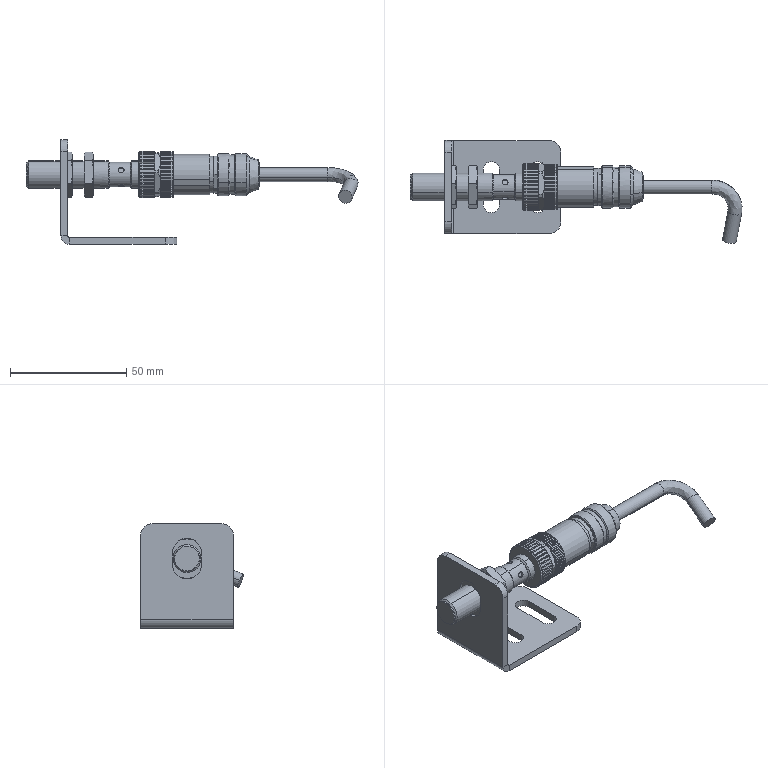Part | SolidWorks | 3 solids | 690 faces | box 143.072 x 44.348 x 45 mm | volume 25932 mm3 | plane 368 | cylinder 200 | cone 120 | spline 2 | commonest cylinder face diameters 19.5 x50 20 x38 2.5 x12 12 x10 1 x8 1.1 x8